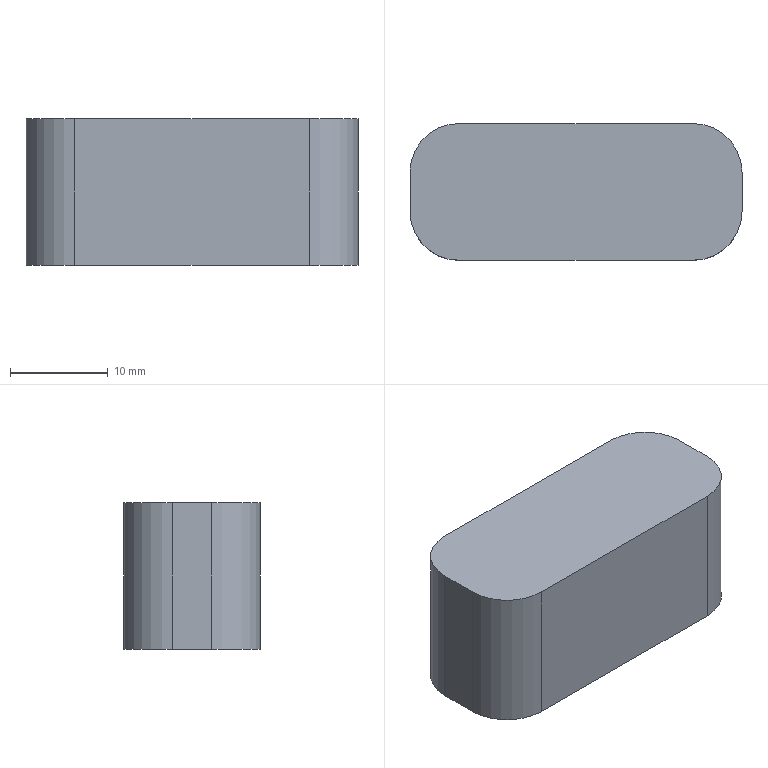Part | SolidWorks | features BaseBody 1 | 1 solid | 10 faces | box 34 x 14 x 15 mm | volume 6818 mm3 | plane 6 | cylinder 4 | commonest cylinder face diameters 10 x4
STEP:
#1=CARTESIAN_POINT('',(12.,-7.,0.));
#2=VERTEX_POINT('',#1);
#3=CARTESIAN_POINT('',(17.,-2.,0.));
#4=VERTEX_POINT('',#3);
#5=CARTESIAN_POINT('',(12.,-2.,0.));
#6=DIRECTION('',(0.,0.,1.));
#7=DIRECTION('',(-1.,0.,0.));
#8=AXIS2_PLACEMENT_3D('',#5,#6,#7);
#9=CIRCLE('',#8,5.);
#10=EDGE_CURVE('',#2,#4,#9,.T.);
#11=ORIENTED_EDGE('',*,*,#10,.F.);
#12=CARTESIAN_POINT('',(-12.,-7.,0.));
#13=VERTEX_POINT('',#12);
#14=CARTESIAN_POINT('',(0.,-7.,0.));
#15=DIRECTION('',(1.,0.,0.));
#16=VECTOR('',#15,1000.);
#17=LINE('',#14,#16);
#18=EDGE_CURVE('',#13,#2,#17,.T.);
#19=ORIENTED_EDGE('',*,*,#18,.F.);
#20=CARTESIAN_POINT('',(-17.,-2.,0.));
#21=VERTEX_POINT('',#20);
#22=CARTESIAN_POINT('',(-12.,-2.,0.));
#23=DIRECTION('',(0.,0.,1.));
#24=DIRECTION('',(-1.,0.,0.));
#25=AXIS2_PLACEMENT_3D('',#22,#23,#24);
#26=CIRCLE('',#25,5.);
#27=EDGE_CURVE('',#21,#13,#26,.T.);
#28=ORIENTED_EDGE('',*,*,#27,.F.);
#29=CARTESIAN_POINT('',(-17.,2.,0.));
#30=VERTEX_POINT('',#29);
#31=CARTESIAN_POINT('',(-17.,0.,0.));
#32=DIRECTION('',(0.,-1.,0.));
#33=VECTOR('',#32,1000.);
#34=LINE('',#31,#33);
#35=EDGE_CURVE('',#30,#21,#34,.T.);
#36=ORIENTED_EDGE('',*,*,#35,.F.);
#37=CARTESIAN_POINT('',(-12.,7.,0.));
#38=VERTEX_POINT('',#37);
#39=CARTESIAN_POINT('',(-12.,2.,0.));
#40=DIRECTION('',(0.,0.,1.));
#41=DIRECTION('',(-1.,0.,0.));
#42=AXIS2_PLACEMENT_3D('',#39,#40,#41);
#43=CIRCLE('',#42,5.);
#44=EDGE_CURVE('',#38,#30,#43,.T.);
#45=ORIENTED_EDGE('',*,*,#44,.F.);
#46=CARTESIAN_POINT('',(12.,7.,0.));
#47=VERTEX_POINT('',#46);
#48=CARTESIAN_POINT('',(0.,7.,0.));
#49=DIRECTION('',(-1.,0.,0.));
#50=VECTOR('',#49,1000.);
#51=LINE('',#48,#50);
#52=EDGE_CURVE('',#47,#38,#51,.T.);
#53=ORIENTED_EDGE('',*,*,#52,.F.);
#54=CARTESIAN_POINT('',(17.,2.,0.));
#55=VERTEX_POINT('',#54);
#56=CARTESIAN_POINT('',(12.,2.,0.));
#57=DIRECTION('',(0.,0.,1.));
#58=DIRECTION('',(-1.,0.,0.));
#59=AXIS2_PLACEMENT_3D('',#56,#57,#58);
#60=CIRCLE('',#59,5.);
#61=EDGE_CURVE('',#55,#47,#60,.T.);
#62=ORIENTED_EDGE('',*,*,#61,.F.);
#63=CARTESIAN_POINT('',(17.,0.,0.));
#64=DIRECTION('',(0.,1.,0.));
#65=VECTOR('',#64,1000.);
#66=LINE('',#63,#65);
#67=EDGE_CURVE('',#4,#55,#66,.T.);
#68=ORIENTED_EDGE('',*,*,#67,.F.);
#69=EDGE_LOOP('',(#11,#19,#28,#36,#45,#53,#62,#68));
#70=FACE_OUTER_BOUND('',#69,.T.);
#71=CARTESIAN_POINT('',(0.,0.,0.));
#72=DIRECTION('',(0.,0.,1.));
#73=DIRECTION('',(1.,0.,0.));
#74=AXIS2_PLACEMENT_3D('',#71,#72,#73);
#75=PLANE('',#74);
#76=ADVANCED_FACE('',(#70),#75,.F.);
#77=CARTESIAN_POINT('',(17.,-2.,15.));
#78=VERTEX_POINT('',#77);
#79=CARTESIAN_POINT('',(17.,-2.,15.));
#80=DIRECTION('',(0.,0.,1.));
#81=VECTOR('',#80,1000.);
#82=LINE('',#79,#81);
#83=EDGE_CURVE('',#4,#78,#82,.T.);
#84=ORIENTED_EDGE('',*,*,#83,.F.);
#85=ORIENTED_EDGE('',*,*,#67,.T.);
#86=CARTESIAN_POINT('',(17.,2.,15.));
#87=VERTEX_POINT('',#86);
#88=CARTESIAN_POINT('',(17.,2.,15.));
#89=DIRECTION('',(0.,0.,-1.));
#90=VECTOR('',#89,1000.);
#91=LINE('',#88,#90);
#92=EDGE_CURVE('',#87,#55,#91,.T.);
#93=ORIENTED_EDGE('',*,*,#92,.F.);
#94=CARTESIAN_POINT('',(17.,7.,15.));
#95=DIRECTION('',(0.,1.,0.));
#96=VECTOR('',#95,1000.);
#97=LINE('',#94,#96);
#98=EDGE_CURVE('',#78,#87,#97,.T.);
#99=ORIENTED_EDGE('',*,*,#98,.F.);
#100=EDGE_LOOP('',(#84,#85,#93,#99));
#101=FACE_OUTER_BOUND('',#100,.T.);
#102=CARTESIAN_POINT('',(17.,7.,15.));
#103=DIRECTION('',(-1.,0.,0.));
#104=DIRECTION('',(0.,0.,1.));
#105=AXIS2_PLACEMENT_3D('',#102,#103,#104);
#106=PLANE('',#105);
#107=ADVANCED_FACE('',(#101),#106,.F.);
#108=ORIENTED_EDGE('',*,*,#10,.T.);
#109=ORIENTED_EDGE('',*,*,#83,.T.);
#110=CARTESIAN_POINT('',(12.,-7.,15.));
#111=VERTEX_POINT('',#110);
#112=CARTESIAN_POINT('',(12.,-2.,15.));
#113=DIRECTION('',(0.,0.,-1.));
#114=DIRECTION('',(-1.,0.,0.));
#115=AXIS2_PLACEMENT_3D('',#112,#113,#114);
#116=CIRCLE('',#115,5.);
#117=EDGE_CURVE('',#78,#111,#116,.T.);
#118=ORIENTED_EDGE('',*,*,#117,.T.);
#119=CARTESIAN_POINT('',(12.,-7.,15.));
#120=DIRECTION('',(0.,0.,-1.));
#121=VECTOR('',#120,1000.);
#122=LINE('',#119,#121);
#123=EDGE_CURVE('',#111,#2,#122,.T.);
#124=ORIENTED_EDGE('',*,*,#123,.T.);
#125=EDGE_LOOP('',(#108,#109,#118,#124));
#126=FACE_OUTER_BOUND('',#125,.T.);
#127=CARTESIAN_POINT('',(12.,-2.,15.));
#128=DIRECTION('',(0.,0.,-1.));
#129=DIRECTION('',(-1.,0.,0.));
#130=AXIS2_PLACEMENT_3D('',#127,#128,#129);
#131=CYLINDRICAL_SURFACE('',#130,5.);
#132=ADVANCED_FACE('',(#126),#131,.T.);
#133=ORIENTED_EDGE('',*,*,#123,.F.);
#134=CARTESIAN_POINT('',(-12.,-7.,15.));
#135=VERTEX_POINT('',#134);
#136=CARTESIAN_POINT('',(-17.,-7.,15.));
#137=DIRECTION('',(1.,0.,0.));
#138=VECTOR('',#137,1000.);
#139=LINE('',#136,#138);
#140=EDGE_CURVE('',#135,#111,#139,.T.);
#141=ORIENTED_EDGE('',*,*,#140,.F.);
#142=CARTESIAN_POINT('',(-12.,-7.,15.));
#143=DIRECTION('',(0.,0.,1.));
#144=VECTOR('',#143,1000.);
#145=LINE('',#142,#144);
#146=EDGE_CURVE('',#13,#135,#145,.T.);
#147=ORIENTED_EDGE('',*,*,#146,.F.);
#148=ORIENTED_EDGE('',*,*,#18,.T.);
#149=EDGE_LOOP('',(#133,#141,#147,#148));
#150=FACE_OUTER_BOUND('',#149,.T.);
#151=CARTESIAN_POINT('',(-17.,-7.,15.));
#152=DIRECTION('',(0.,1.,0.));
#153=DIRECTION('',(0.,0.,1.));
#154=AXIS2_PLACEMENT_3D('',#151,#152,#153);
#155=PLANE('',#154);
#156=ADVANCED_FACE('',(#150),#155,.F.);
#157=ORIENTED_EDGE('',*,*,#27,.T.);
#158=ORIENTED_EDGE('',*,*,#146,.T.);
#159=CARTESIAN_POINT('',(-17.,-2.,15.));
#160=VERTEX_POINT('',#159);
#161=CARTESIAN_POINT('',(-12.,-2.,15.));
#162=DIRECTION('',(0.,0.,-1.));
#163=DIRECTION('',(-1.,0.,0.));
#164=AXIS2_PLACEMENT_3D('',#161,#162,#163);
#165=CIRCLE('',#164,5.);
#166=EDGE_CURVE('',#135,#160,#165,.T.);
#167=ORIENTED_EDGE('',*,*,#166,.T.);
#168=CARTESIAN_POINT('',(-17.,-2.,15.));
#169=DIRECTION('',(0.,0.,-1.));
#170=VECTOR('',#169,1000.);
#171=LINE('',#168,#170);
#172=EDGE_CURVE('',#160,#21,#171,.T.);
#173=ORIENTED_EDGE('',*,*,#172,.T.);
#174=EDGE_LOOP('',(#157,#158,#167,#173));
#175=FACE_OUTER_BOUND('',#174,.T.);
#176=CARTESIAN_POINT('',(-12.,-2.,15.));
#177=DIRECTION('',(0.,0.,-1.));
#178=DIRECTION('',(-1.,0.,0.));
#179=AXIS2_PLACEMENT_3D('',#176,#177,#178);
#180=CYLINDRICAL_SURFACE('',#179,5.);
#181=ADVANCED_FACE('',(#175),#180,.T.);
#182=ORIENTED_EDGE('',*,*,#172,.F.);
#183=CARTESIAN_POINT('',(-17.,2.,15.));
#184=VERTEX_POINT('',#183);
#185=CARTESIAN_POINT('',(-17.,7.,15.));
#186=DIRECTION('',(0.,-1.,0.));
#187=VECTOR('',#186,1000.);
#188=LINE('',#185,#187);
#189=EDGE_CURVE('',#184,#160,#188,.T.);
#190=ORIENTED_EDGE('',*,*,#189,.F.);
#191=CARTESIAN_POINT('',(-17.,2.,15.));
#192=DIRECTION('',(0.,0.,1.));
#193=VECTOR('',#192,1000.);
#194=LINE('',#191,#193);
#195=EDGE_CURVE('',#30,#184,#194,.T.);
#196=ORIENTED_EDGE('',*,*,#195,.F.);
#197=ORIENTED_EDGE('',*,*,#35,.T.);
#198=EDGE_LOOP('',(#182,#190,#196,#197));
#199=FACE_OUTER_BOUND('',#198,.T.);
#200=CARTESIAN_POINT('',(-17.,7.,15.));
#201=DIRECTION('',(1.,0.,0.));
#202=DIRECTION('',(0.,1.,0.));
#203=AXIS2_PLACEMENT_3D('',#200,#201,#202);
#204=PLANE('',#203);
#205=ADVANCED_FACE('',(#199),#204,.F.);
#206=ORIENTED_EDGE('',*,*,#44,.T.);
#207=ORIENTED_EDGE('',*,*,#195,.T.);
#208=CARTESIAN_POINT('',(-12.,7.,15.));
#209=VERTEX_POINT('',#208);
#210=CARTESIAN_POINT('',(-12.,2.,15.));
#211=DIRECTION('',(0.,0.,-1.));
#212=DIRECTION('',(-1.,0.,0.));
#213=AXIS2_PLACEMENT_3D('',#210,#211,#212);
#214=CIRCLE('',#213,5.);
#215=EDGE_CURVE('',#184,#209,#214,.T.);
#216=ORIENTED_EDGE('',*,*,#215,.T.);
#217=CARTESIAN_POINT('',(-12.,7.,15.));
#218=DIRECTION('',(0.,0.,-1.));
#219=VECTOR('',#218,1000.);
#220=LINE('',#217,#219);
#221=EDGE_CURVE('',#209,#38,#220,.T.);
#222=ORIENTED_EDGE('',*,*,#221,.T.);
#223=EDGE_LOOP('',(#206,#207,#216,#222));
#224=FACE_OUTER_BOUND('',#223,.T.);
#225=CARTESIAN_POINT('',(-12.,2.,15.));
#226=DIRECTION('',(0.,0.,-1.));
#227=DIRECTION('',(-1.,0.,0.));
#228=AXIS2_PLACEMENT_3D('',#225,#226,#227);
#229=CYLINDRICAL_SURFACE('',#228,5.);
#230=ADVANCED_FACE('',(#224),#229,.T.);
#231=CARTESIAN_POINT('',(12.,7.,15.));
#232=VERTEX_POINT('',#231);
#233=CARTESIAN_POINT('',(12.,7.,15.));
#234=DIRECTION('',(0.,0.,1.));
#235=VECTOR('',#234,1000.);
#236=LINE('',#233,#235);
#237=EDGE_CURVE('',#47,#232,#236,.T.);
#238=ORIENTED_EDGE('',*,*,#237,.F.);
#239=ORIENTED_EDGE('',*,*,#52,.T.);
#240=ORIENTED_EDGE('',*,*,#221,.F.);
#241=CARTESIAN_POINT('',(-17.,7.,15.));
#242=DIRECTION('',(-1.,0.,0.));
#243=VECTOR('',#242,1000.);
#244=LINE('',#241,#243);
#245=EDGE_CURVE('',#232,#209,#244,.T.);
#246=ORIENTED_EDGE('',*,*,#245,.F.);
#247=EDGE_LOOP('',(#238,#239,#240,#246));
#248=FACE_OUTER_BOUND('',#247,.T.);
#249=CARTESIAN_POINT('',(-17.,7.,15.));
#250=DIRECTION('',(0.,-1.,0.));
#251=DIRECTION('',(0.,0.,-1.));
#252=AXIS2_PLACEMENT_3D('',#249,#250,#251);
#253=PLANE('',#252);
#254=ADVANCED_FACE('',(#248),#253,.F.);
#255=ORIENTED_EDGE('',*,*,#61,.T.);
#256=ORIENTED_EDGE('',*,*,#237,.T.);
#257=CARTESIAN_POINT('',(12.,2.,15.));
#258=DIRECTION('',(0.,0.,-1.));
#259=DIRECTION('',(-1.,0.,0.));
#260=AXIS2_PLACEMENT_3D('',#257,#258,#259);
#261=CIRCLE('',#260,5.);
#262=EDGE_CURVE('',#232,#87,#261,.T.);
#263=ORIENTED_EDGE('',*,*,#262,.T.);
#264=ORIENTED_EDGE('',*,*,#92,.T.);
#265=EDGE_LOOP('',(#255,#256,#263,#264));
#266=FACE_OUTER_BOUND('',#265,.T.);
#267=CARTESIAN_POINT('',(12.,2.,15.));
#268=DIRECTION('',(0.,0.,-1.));
#269=DIRECTION('',(-1.,0.,0.));
#270=AXIS2_PLACEMENT_3D('',#267,#268,#269);
#271=CYLINDRICAL_SURFACE('',#270,5.);
#272=ADVANCED_FACE('',(#266),#271,.T.);
#273=ORIENTED_EDGE('',*,*,#189,.T.);
#274=ORIENTED_EDGE('',*,*,#166,.F.);
#275=ORIENTED_EDGE('',*,*,#140,.T.);
#276=ORIENTED_EDGE('',*,*,#117,.F.);
#277=ORIENTED_EDGE('',*,*,#98,.T.);
#278=ORIENTED_EDGE('',*,*,#262,.F.);
#279=ORIENTED_EDGE('',*,*,#245,.T.);
#280=ORIENTED_EDGE('',*,*,#215,.F.);
#281=EDGE_LOOP('',(#273,#274,#275,#276,#277,#278,#279,#280));
#282=FACE_OUTER_BOUND('',#281,.T.);
#283=CARTESIAN_POINT('',(0.,0.,15.));
#284=DIRECTION('',(0.,0.,1.));
#285=DIRECTION('',(1.,0.,0.));
#286=AXIS2_PLACEMENT_3D('',#283,#284,#285);
#287=PLANE('',#286);
#288=ADVANCED_FACE('',(#282),#287,.T.);
#289=CLOSED_SHELL('',(#76,#107,#132,#156,#181,#205,#230,#254,#272,#288));
#290=MANIFOLD_SOLID_BREP('',#289);
#291=CARTESIAN_POINT('',(0.,0.,0.));
#292=DIRECTION('',(0.,0.,1.));
#293=DIRECTION('',(1.,0.,0.));
#294=AXIS2_PLACEMENT_3D('',#291,#292,#293);
#295=(LENGTH_UNIT()NAMED_UNIT(*)SI_UNIT(.MILLI.,.METRE.));
#296=UNCERTAINTY_MEASURE_WITH_UNIT(LENGTH_MEASURE(0.00001),#295,'','');
#297=(NAMED_UNIT(*)PLANE_ANGLE_UNIT()SI_UNIT($,.RADIAN.));
#298=(NAMED_UNIT(*)SI_UNIT($,.STERADIAN.)SOLID_ANGLE_UNIT());
#299=(GEOMETRIC_REPRESENTATION_CONTEXT(3)GLOBAL_UNCERTAINTY_ASSIGNED_CONTEXT((#296))GLOBAL_UNIT_ASSIGNED_CONTEXT((#295,#297,#298))REPRESENTATION_CONTEXT('',''));
#300=ADVANCED_BREP_SHAPE_REPRESENTATION('',(#290,#294),#299);